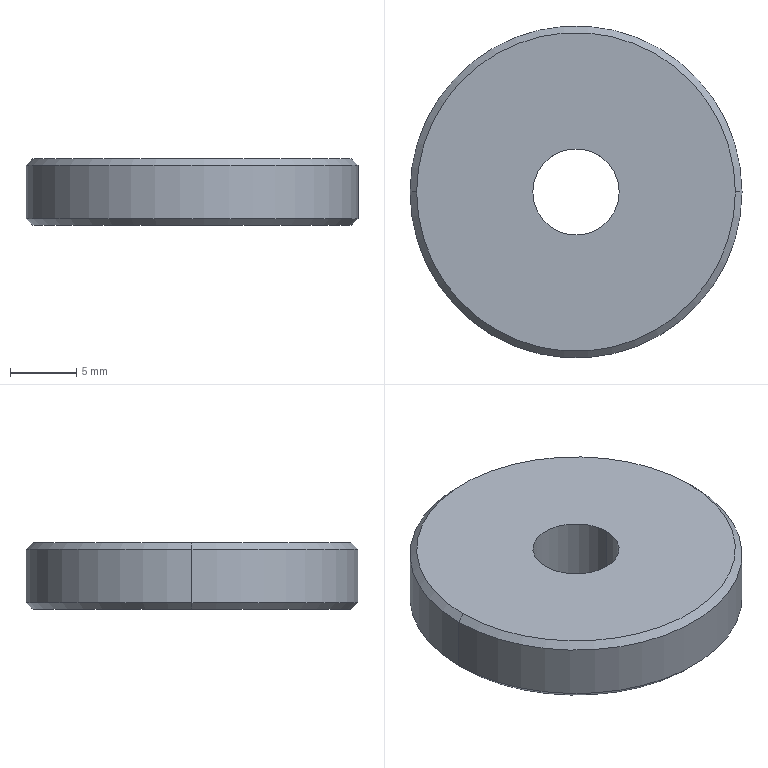Part | SolidWorks | features Chamfer 1, Extrusion 1 | 1 solid | 10 faces | box 25 x 25 x 5 mm | volume 2269 mm3 | cone 4 | cylinder 4 | plane 2 | commonest cylinder face diameters 6.5 x2 25 x2
STEP:
#1=CARTESIAN_POINT('',(12.,0.,2.5));
#2=VERTEX_POINT('',#1);
#3=CARTESIAN_POINT('',(-12.,0.,2.5));
#4=VERTEX_POINT('',#3);
#5=CARTESIAN_POINT('',(0.,0.,2.5));
#6=DIRECTION('',(0.,0.,1.));
#7=DIRECTION('',(1.,0.,0.));
#8=AXIS2_PLACEMENT_3D('',#5,#6,#7);
#9=CIRCLE('',#8,12.);
#10=EDGE_CURVE('',#2,#4,#9,.T.);
#11=ORIENTED_EDGE('',*,*,#10,.F.);
#12=CARTESIAN_POINT('',(12.5,0.,2.));
#13=VERTEX_POINT('',#12);
#14=CARTESIAN_POINT('',(12.,0.,2.5));
#15=DIRECTION('',(0.7071,0.,-0.7071));
#16=VECTOR('',#15,1000.);
#17=LINE('',#14,#16);
#18=EDGE_CURVE('',#2,#13,#17,.T.);
#19=ORIENTED_EDGE('',*,*,#18,.T.);
#20=CARTESIAN_POINT('',(-12.5,0.,2.));
#21=VERTEX_POINT('',#20);
#22=CARTESIAN_POINT('',(0.,0.,2.));
#23=DIRECTION('',(0.,0.,-1.));
#24=DIRECTION('',(1.,0.,0.));
#25=AXIS2_PLACEMENT_3D('',#22,#23,#24);
#26=CIRCLE('',#25,12.5);
#27=EDGE_CURVE('',#21,#13,#26,.T.);
#28=ORIENTED_EDGE('',*,*,#27,.F.);
#29=CARTESIAN_POINT('',(-12.,0.,2.5));
#30=DIRECTION('',(-0.7071,0.,-0.7071));
#31=VECTOR('',#30,1000.);
#32=LINE('',#29,#31);
#33=EDGE_CURVE('',#4,#21,#32,.T.);
#34=ORIENTED_EDGE('',*,*,#33,.F.);
#35=EDGE_LOOP('',(#11,#19,#28,#34));
#36=FACE_OUTER_BOUND('',#35,.T.);
#37=CARTESIAN_POINT('',(0.,0.,2.5));
#38=DIRECTION('',(0.,0.,-1.));
#39=DIRECTION('',(-1.,0.,0.));
#40=AXIS2_PLACEMENT_3D('',#37,#38,#39);
#41=CONICAL_SURFACE('',#40,12.,0.7854);
#42=ADVANCED_FACE('',(#36),#41,.T.);
#43=CARTESIAN_POINT('',(-12.,0.,-2.5));
#44=VERTEX_POINT('',#43);
#45=CARTESIAN_POINT('',(12.,0.,-2.5));
#46=VERTEX_POINT('',#45);
#47=CARTESIAN_POINT('',(0.,0.,-2.5));
#48=DIRECTION('',(0.,0.,-1.));
#49=DIRECTION('',(1.,0.,0.));
#50=AXIS2_PLACEMENT_3D('',#47,#48,#49);
#51=CIRCLE('',#50,12.);
#52=EDGE_CURVE('',#44,#46,#51,.T.);
#53=ORIENTED_EDGE('',*,*,#52,.F.);
#54=CARTESIAN_POINT('',(-12.5,0.,-2.));
#55=VERTEX_POINT('',#54);
#56=CARTESIAN_POINT('',(-12.5,0.,-2.));
#57=DIRECTION('',(-0.7071,0.,0.7071));
#58=VECTOR('',#57,1000.);
#59=LINE('',#56,#58);
#60=EDGE_CURVE('',#44,#55,#59,.T.);
#61=ORIENTED_EDGE('',*,*,#60,.T.);
#62=CARTESIAN_POINT('',(12.5,0.,-2.));
#63=VERTEX_POINT('',#62);
#64=CARTESIAN_POINT('',(0.,0.,-2.));
#65=DIRECTION('',(0.,0.,1.));
#66=DIRECTION('',(1.,0.,0.));
#67=AXIS2_PLACEMENT_3D('',#64,#65,#66);
#68=CIRCLE('',#67,12.5);
#69=EDGE_CURVE('',#63,#55,#68,.T.);
#70=ORIENTED_EDGE('',*,*,#69,.F.);
#71=CARTESIAN_POINT('',(12.5,0.,-2.));
#72=DIRECTION('',(0.7071,0.,0.7071));
#73=VECTOR('',#72,1000.);
#74=LINE('',#71,#73);
#75=EDGE_CURVE('',#46,#63,#74,.T.);
#76=ORIENTED_EDGE('',*,*,#75,.F.);
#77=EDGE_LOOP('',(#53,#61,#70,#76));
#78=FACE_OUTER_BOUND('',#77,.T.);
#79=CARTESIAN_POINT('',(0.,0.,-2.));
#80=DIRECTION('',(0.,0.,1.));
#81=DIRECTION('',(1.,0.,0.));
#82=AXIS2_PLACEMENT_3D('',#79,#80,#81);
#83=CONICAL_SURFACE('',#82,12.5,0.7854);
#84=ADVANCED_FACE('',(#78),#83,.T.);
#85=CARTESIAN_POINT('',(-3.25,0.,2.5));
#86=VERTEX_POINT('',#85);
#87=CARTESIAN_POINT('',(3.25,0.,2.5));
#88=VERTEX_POINT('',#87);
#89=CARTESIAN_POINT('',(0.,0.,2.5));
#90=DIRECTION('',(0.,0.,1.));
#91=DIRECTION('',(1.,0.,0.));
#92=AXIS2_PLACEMENT_3D('',#89,#90,#91);
#93=CIRCLE('',#92,3.25);
#94=EDGE_CURVE('',#86,#88,#93,.T.);
#95=ORIENTED_EDGE('',*,*,#94,.T.);
#96=CARTESIAN_POINT('',(3.25,0.,-2.5));
#97=VERTEX_POINT('',#96);
#98=CARTESIAN_POINT('',(3.25,0.,2.5));
#99=DIRECTION('',(0.,0.,-1.));
#100=VECTOR('',#99,1000.);
#101=LINE('',#98,#100);
#102=EDGE_CURVE('',#88,#97,#101,.T.);
#103=ORIENTED_EDGE('',*,*,#102,.T.);
#104=CARTESIAN_POINT('',(-3.25,0.,-2.5));
#105=VERTEX_POINT('',#104);
#106=CARTESIAN_POINT('',(0.,0.,-2.5));
#107=DIRECTION('',(0.,0.,1.));
#108=DIRECTION('',(1.,0.,0.));
#109=AXIS2_PLACEMENT_3D('',#106,#107,#108);
#110=CIRCLE('',#109,3.25);
#111=EDGE_CURVE('',#105,#97,#110,.T.);
#112=ORIENTED_EDGE('',*,*,#111,.F.);
#113=CARTESIAN_POINT('',(-3.25,0.,2.5));
#114=DIRECTION('',(0.,0.,-1.));
#115=VECTOR('',#114,1000.);
#116=LINE('',#113,#115);
#117=EDGE_CURVE('',#86,#105,#116,.T.);
#118=ORIENTED_EDGE('',*,*,#117,.F.);
#119=EDGE_LOOP('',(#95,#103,#112,#118));
#120=FACE_OUTER_BOUND('',#119,.T.);
#121=CARTESIAN_POINT('',(0.,0.,2.5));
#122=DIRECTION('',(0.,0.,-1.));
#123=DIRECTION('',(-1.,0.,0.));
#124=AXIS2_PLACEMENT_3D('',#121,#122,#123);
#125=CYLINDRICAL_SURFACE('',#124,3.25);
#126=ADVANCED_FACE('',(#120),#125,.F.);
#127=ORIENTED_EDGE('',*,*,#27,.T.);
#128=CARTESIAN_POINT('',(12.5,0.,2.5));
#129=DIRECTION('',(0.,0.,-1.));
#130=VECTOR('',#129,1000.);
#131=LINE('',#128,#130);
#132=EDGE_CURVE('',#13,#63,#131,.T.);
#133=ORIENTED_EDGE('',*,*,#132,.T.);
#134=ORIENTED_EDGE('',*,*,#69,.T.);
#135=CARTESIAN_POINT('',(-12.5,0.,2.5));
#136=DIRECTION('',(0.,0.,-1.));
#137=VECTOR('',#136,1000.);
#138=LINE('',#135,#137);
#139=EDGE_CURVE('',#21,#55,#138,.T.);
#140=ORIENTED_EDGE('',*,*,#139,.F.);
#141=EDGE_LOOP('',(#127,#133,#134,#140));
#142=FACE_OUTER_BOUND('',#141,.T.);
#143=CARTESIAN_POINT('',(0.,0.,2.5));
#144=DIRECTION('',(0.,0.,-1.));
#145=DIRECTION('',(-1.,0.,0.));
#146=AXIS2_PLACEMENT_3D('',#143,#144,#145);
#147=CYLINDRICAL_SURFACE('',#146,12.5);
#148=ADVANCED_FACE('',(#142),#147,.T.);
#149=CARTESIAN_POINT('',(0.,0.,2.5));
#150=DIRECTION('',(0.,0.,1.));
#151=DIRECTION('',(1.,0.,0.));
#152=AXIS2_PLACEMENT_3D('',#149,#150,#151);
#153=CIRCLE('',#152,12.);
#154=EDGE_CURVE('',#4,#2,#153,.T.);
#155=ORIENTED_EDGE('',*,*,#154,.T.);
#156=ORIENTED_EDGE('',*,*,#10,.T.);
#157=EDGE_LOOP('',(#155,#156));
#158=FACE_OUTER_BOUND('',#157,.T.);
#159=ORIENTED_EDGE('',*,*,#94,.F.);
#160=CARTESIAN_POINT('',(0.,0.,2.5));
#161=DIRECTION('',(0.,0.,1.));
#162=DIRECTION('',(1.,0.,0.));
#163=AXIS2_PLACEMENT_3D('',#160,#161,#162);
#164=CIRCLE('',#163,3.25);
#165=EDGE_CURVE('',#88,#86,#164,.T.);
#166=ORIENTED_EDGE('',*,*,#165,.F.);
#167=EDGE_LOOP('',(#159,#166));
#168=FACE_BOUND('',#167,.T.);
#169=CARTESIAN_POINT('',(0.,0.,2.5));
#170=DIRECTION('',(0.,0.,1.));
#171=DIRECTION('',(1.,0.,0.));
#172=AXIS2_PLACEMENT_3D('',#169,#170,#171);
#173=PLANE('',#172);
#174=ADVANCED_FACE('',(#158,#168),#173,.T.);
#175=CARTESIAN_POINT('',(0.,0.,-2.5));
#176=DIRECTION('',(0.,0.,-1.));
#177=DIRECTION('',(1.,0.,0.));
#178=AXIS2_PLACEMENT_3D('',#175,#176,#177);
#179=CIRCLE('',#178,12.);
#180=EDGE_CURVE('',#46,#44,#179,.T.);
#181=ORIENTED_EDGE('',*,*,#180,.T.);
#182=ORIENTED_EDGE('',*,*,#52,.T.);
#183=EDGE_LOOP('',(#181,#182));
#184=FACE_OUTER_BOUND('',#183,.T.);
#185=ORIENTED_EDGE('',*,*,#111,.T.);
#186=CARTESIAN_POINT('',(0.,0.,-2.5));
#187=DIRECTION('',(0.,0.,1.));
#188=DIRECTION('',(1.,0.,0.));
#189=AXIS2_PLACEMENT_3D('',#186,#187,#188);
#190=CIRCLE('',#189,3.25);
#191=EDGE_CURVE('',#97,#105,#190,.T.);
#192=ORIENTED_EDGE('',*,*,#191,.T.);
#193=EDGE_LOOP('',(#185,#192));
#194=FACE_BOUND('',#193,.T.);
#195=CARTESIAN_POINT('',(0.,0.,-2.5));
#196=DIRECTION('',(0.,0.,1.));
#197=DIRECTION('',(1.,0.,0.));
#198=AXIS2_PLACEMENT_3D('',#195,#196,#197);
#199=PLANE('',#198);
#200=ADVANCED_FACE('',(#184,#194),#199,.F.);
#201=ORIENTED_EDGE('',*,*,#132,.F.);
#202=CARTESIAN_POINT('',(0.,0.,2.));
#203=DIRECTION('',(0.,0.,-1.));
#204=DIRECTION('',(1.,0.,0.));
#205=AXIS2_PLACEMENT_3D('',#202,#203,#204);
#206=CIRCLE('',#205,12.5);
#207=EDGE_CURVE('',#13,#21,#206,.T.);
#208=ORIENTED_EDGE('',*,*,#207,.T.);
#209=ORIENTED_EDGE('',*,*,#139,.T.);
#210=CARTESIAN_POINT('',(0.,0.,-2.));
#211=DIRECTION('',(0.,0.,1.));
#212=DIRECTION('',(1.,0.,0.));
#213=AXIS2_PLACEMENT_3D('',#210,#211,#212);
#214=CIRCLE('',#213,12.5);
#215=EDGE_CURVE('',#55,#63,#214,.T.);
#216=ORIENTED_EDGE('',*,*,#215,.T.);
#217=EDGE_LOOP('',(#201,#208,#209,#216));
#218=FACE_OUTER_BOUND('',#217,.T.);
#219=CARTESIAN_POINT('',(0.,0.,2.5));
#220=DIRECTION('',(0.,0.,-1.));
#221=DIRECTION('',(-1.,0.,0.));
#222=AXIS2_PLACEMENT_3D('',#219,#220,#221);
#223=CYLINDRICAL_SURFACE('',#222,12.5);
#224=ADVANCED_FACE('',(#218),#223,.T.);
#225=ORIENTED_EDGE('',*,*,#102,.F.);
#226=ORIENTED_EDGE('',*,*,#165,.T.);
#227=ORIENTED_EDGE('',*,*,#117,.T.);
#228=ORIENTED_EDGE('',*,*,#191,.F.);
#229=EDGE_LOOP('',(#225,#226,#227,#228));
#230=FACE_OUTER_BOUND('',#229,.T.);
#231=CARTESIAN_POINT('',(0.,0.,2.5));
#232=DIRECTION('',(0.,0.,-1.));
#233=DIRECTION('',(-1.,0.,0.));
#234=AXIS2_PLACEMENT_3D('',#231,#232,#233);
#235=CYLINDRICAL_SURFACE('',#234,3.25);
#236=ADVANCED_FACE('',(#230),#235,.F.);
#237=ORIENTED_EDGE('',*,*,#60,.F.);
#238=ORIENTED_EDGE('',*,*,#180,.F.);
#239=ORIENTED_EDGE('',*,*,#75,.T.);
#240=ORIENTED_EDGE('',*,*,#215,.F.);
#241=EDGE_LOOP('',(#237,#238,#239,#240));
#242=FACE_OUTER_BOUND('',#241,.T.);
#243=CARTESIAN_POINT('',(0.,0.,-2.));
#244=DIRECTION('',(0.,0.,1.));
#245=DIRECTION('',(1.,0.,0.));
#246=AXIS2_PLACEMENT_3D('',#243,#244,#245);
#247=CONICAL_SURFACE('',#246,12.5,0.7854);
#248=ADVANCED_FACE('',(#242),#247,.T.);
#249=ORIENTED_EDGE('',*,*,#18,.F.);
#250=ORIENTED_EDGE('',*,*,#154,.F.);
#251=ORIENTED_EDGE('',*,*,#33,.T.);
#252=ORIENTED_EDGE('',*,*,#207,.F.);
#253=EDGE_LOOP('',(#249,#250,#251,#252));
#254=FACE_OUTER_BOUND('',#253,.T.);
#255=CARTESIAN_POINT('',(0.,0.,2.5));
#256=DIRECTION('',(0.,0.,-1.));
#257=DIRECTION('',(-1.,0.,0.));
#258=AXIS2_PLACEMENT_3D('',#255,#256,#257);
#259=CONICAL_SURFACE('',#258,12.,0.7854);
#260=ADVANCED_FACE('',(#254),#259,.T.);
#261=CLOSED_SHELL('',(#42,#84,#126,#148,#174,#200,#224,#236,#248,#260));
#262=MANIFOLD_SOLID_BREP('',#261);
#263=CARTESIAN_POINT('',(0.,0.,0.));
#264=DIRECTION('',(0.,0.,1.));
#265=DIRECTION('',(1.,0.,0.));
#266=AXIS2_PLACEMENT_3D('',#263,#264,#265);
#267=(LENGTH_UNIT()NAMED_UNIT(*)SI_UNIT(.MILLI.,.METRE.));
#268=UNCERTAINTY_MEASURE_WITH_UNIT(LENGTH_MEASURE(0.00001),#267,'','');
#269=(NAMED_UNIT(*)PLANE_ANGLE_UNIT()SI_UNIT($,.RADIAN.));
#270=(NAMED_UNIT(*)SI_UNIT($,.STERADIAN.)SOLID_ANGLE_UNIT());
#271=(GEOMETRIC_REPRESENTATION_CONTEXT(3)GLOBAL_UNCERTAINTY_ASSIGNED_CONTEXT((#268))GLOBAL_UNIT_ASSIGNED_CONTEXT((#267,#269,#270))REPRESENTATION_CONTEXT('',''));
#272=ADVANCED_BREP_SHAPE_REPRESENTATION('',(#262,#266),#271);